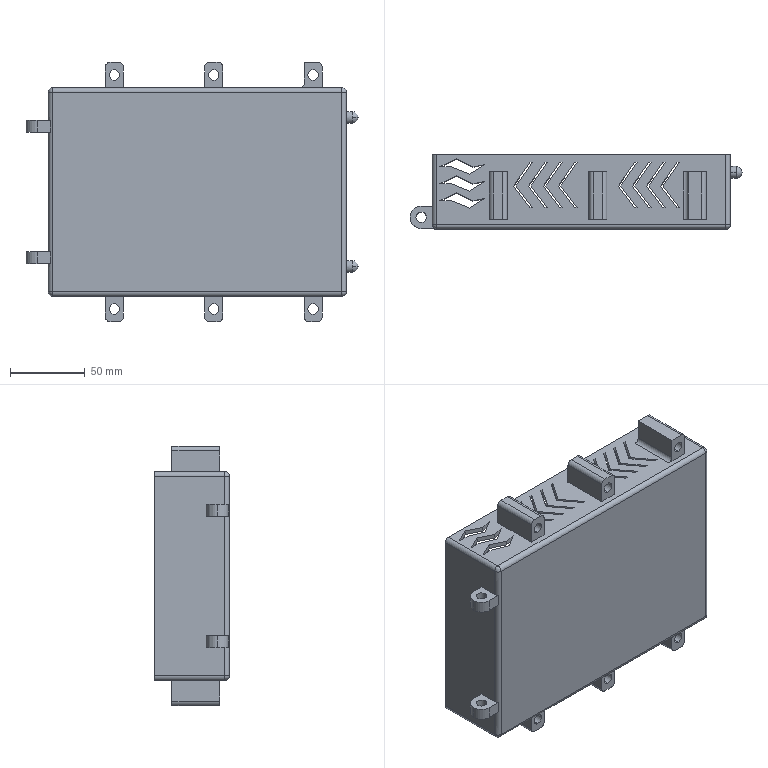Part | SolidWorks | features BaseBody 1 | 1 solid | 244 faces | box 222.738 x 50.026 x 174 mm | volume 466487 mm3 | plane 183 | cylinder 45 | sphere 16 | commonest cylinder face diameters 6 x21 7 x16 8 x4 15 x4